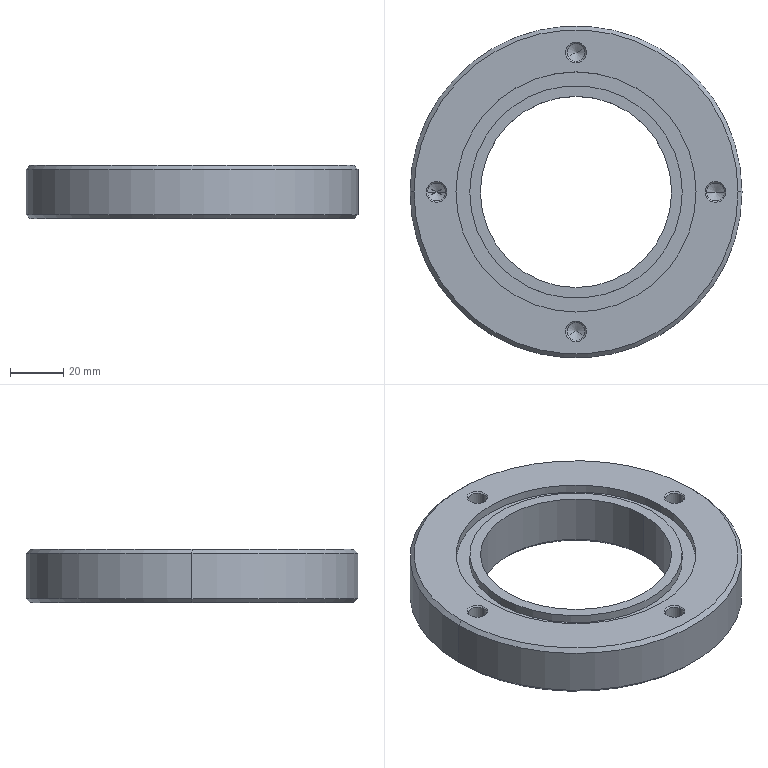Part | SolidWorks | features Chamfer 2, ICE 2, FlatPattern 1, HoleWzd 1, SMBaseFlange 1, SheetMetal 1 | 1 solid | 42 faces | box 125 x 125 x 20 mm | volume 156275 mm3 | cone 22 | cylinder 16 | plane 4 | commonest cylinder face diameters 6.8 x8 72 x2 80 x2 90.4 x2 125 x2
STEP:
#1=CARTESIAN_POINT('',(49.1,0.,-0.5));
#2=VERTEX_POINT('',#1);
#3=CARTESIAN_POINT('',(55.9,0.,-0.5));
#4=VERTEX_POINT('',#3);
#5=CARTESIAN_POINT('',(52.5,0.,-0.5));
#6=DIRECTION('',(0.,0.,1.));
#7=DIRECTION('',(1.,0.,0.));
#8=AXIS2_PLACEMENT_3D('',#5,#6,#7);
#9=CIRCLE('',#8,3.4);
#10=EDGE_CURVE('',#2,#4,#9,.T.);
#11=ORIENTED_EDGE('',*,*,#10,.F.);
#12=CARTESIAN_POINT('',(48.6,0.,0.));
#13=VERTEX_POINT('',#12);
#14=CARTESIAN_POINT('',(49.1,0.,-0.5));
#15=DIRECTION('',(-0.7071,0.,0.7071));
#16=VECTOR('',#15,1000.);
#17=LINE('',#14,#16);
#18=EDGE_CURVE('',#2,#13,#17,.T.);
#19=ORIENTED_EDGE('',*,*,#18,.T.);
#20=CARTESIAN_POINT('',(56.4,0.,0.));
#21=VERTEX_POINT('',#20);
#22=CARTESIAN_POINT('',(52.5,0.,0.));
#23=DIRECTION('',(0.,0.,-1.));
#24=DIRECTION('',(1.,0.,0.));
#25=AXIS2_PLACEMENT_3D('',#22,#23,#24);
#26=CIRCLE('',#25,3.9);
#27=EDGE_CURVE('',#21,#13,#26,.T.);
#28=ORIENTED_EDGE('',*,*,#27,.F.);
#29=CARTESIAN_POINT('',(55.9,0.,-0.5));
#30=DIRECTION('',(0.7071,0.,0.7071));
#31=VECTOR('',#30,1000.);
#32=LINE('',#29,#31);
#33=EDGE_CURVE('',#4,#21,#32,.T.);
#34=ORIENTED_EDGE('',*,*,#33,.F.);
#35=EDGE_LOOP('',(#11,#19,#28,#34));
#36=FACE_OUTER_BOUND('',#35,.T.);
#37=CARTESIAN_POINT('',(52.5,0.,-0.5));
#38=DIRECTION('',(0.,0.,1.));
#39=DIRECTION('',(1.,0.,0.));
#40=AXIS2_PLACEMENT_3D('',#37,#38,#39);
#41=CONICAL_SURFACE('',#40,3.4,0.7854);
#42=ADVANCED_FACE('',(#36),#41,.F.);
#43=CARTESIAN_POINT('',(-3.4,-52.5,-0.5));
#44=VERTEX_POINT('',#43);
#45=CARTESIAN_POINT('',(3.4,-52.5,-0.5));
#46=VERTEX_POINT('',#45);
#47=CARTESIAN_POINT('',(0.,-52.5,-0.5));
#48=DIRECTION('',(0.,0.,1.));
#49=DIRECTION('',(1.,0.,0.));
#50=AXIS2_PLACEMENT_3D('',#47,#48,#49);
#51=CIRCLE('',#50,3.4);
#52=EDGE_CURVE('',#44,#46,#51,.T.);
#53=ORIENTED_EDGE('',*,*,#52,.F.);
#54=CARTESIAN_POINT('',(-3.9,-52.5,0.));
#55=VERTEX_POINT('',#54);
#56=CARTESIAN_POINT('',(-3.4,-52.5,-0.5));
#57=DIRECTION('',(-0.7071,0.,0.7071));
#58=VECTOR('',#57,1000.);
#59=LINE('',#56,#58);
#60=EDGE_CURVE('',#44,#55,#59,.T.);
#61=ORIENTED_EDGE('',*,*,#60,.T.);
#62=CARTESIAN_POINT('',(3.9,-52.5,0.));
#63=VERTEX_POINT('',#62);
#64=CARTESIAN_POINT('',(0.,-52.5,0.));
#65=DIRECTION('',(0.,0.,-1.));
#66=DIRECTION('',(1.,0.,0.));
#67=AXIS2_PLACEMENT_3D('',#64,#65,#66);
#68=CIRCLE('',#67,3.9);
#69=EDGE_CURVE('',#63,#55,#68,.T.);
#70=ORIENTED_EDGE('',*,*,#69,.F.);
#71=CARTESIAN_POINT('',(3.4,-52.5,-0.5));
#72=DIRECTION('',(0.7071,0.,0.7071));
#73=VECTOR('',#72,1000.);
#74=LINE('',#71,#73);
#75=EDGE_CURVE('',#46,#63,#74,.T.);
#76=ORIENTED_EDGE('',*,*,#75,.F.);
#77=EDGE_LOOP('',(#53,#61,#70,#76));
#78=FACE_OUTER_BOUND('',#77,.T.);
#79=CARTESIAN_POINT('',(0.,-52.5,-0.5));
#80=DIRECTION('',(0.,0.,1.));
#81=DIRECTION('',(1.,0.,0.));
#82=AXIS2_PLACEMENT_3D('',#79,#80,#81);
#83=CONICAL_SURFACE('',#82,3.4,0.7854);
#84=ADVANCED_FACE('',(#78),#83,.F.);
#85=CARTESIAN_POINT('',(-55.9,0.,-0.5));
#86=VERTEX_POINT('',#85);
#87=CARTESIAN_POINT('',(-49.1,0.,-0.5));
#88=VERTEX_POINT('',#87);
#89=CARTESIAN_POINT('',(-52.5,0.,-0.5));
#90=DIRECTION('',(0.,0.,1.));
#91=DIRECTION('',(1.,0.,0.));
#92=AXIS2_PLACEMENT_3D('',#89,#90,#91);
#93=CIRCLE('',#92,3.4);
#94=EDGE_CURVE('',#86,#88,#93,.T.);
#95=ORIENTED_EDGE('',*,*,#94,.F.);
#96=CARTESIAN_POINT('',(-56.4,0.,0.));
#97=VERTEX_POINT('',#96);
#98=CARTESIAN_POINT('',(-55.9,0.,-0.5));
#99=DIRECTION('',(-0.7071,0.,0.7071));
#100=VECTOR('',#99,1000.);
#101=LINE('',#98,#100);
#102=EDGE_CURVE('',#86,#97,#101,.T.);
#103=ORIENTED_EDGE('',*,*,#102,.T.);
#104=CARTESIAN_POINT('',(-48.6,0.,0.));
#105=VERTEX_POINT('',#104);
#106=CARTESIAN_POINT('',(-52.5,0.,0.));
#107=DIRECTION('',(0.,0.,-1.));
#108=DIRECTION('',(1.,0.,0.));
#109=AXIS2_PLACEMENT_3D('',#106,#107,#108);
#110=CIRCLE('',#109,3.9);
#111=EDGE_CURVE('',#105,#97,#110,.T.);
#112=ORIENTED_EDGE('',*,*,#111,.F.);
#113=CARTESIAN_POINT('',(-49.1,0.,-0.5));
#114=DIRECTION('',(0.7071,0.,0.7071));
#115=VECTOR('',#114,1000.);
#116=LINE('',#113,#115);
#117=EDGE_CURVE('',#88,#105,#116,.T.);
#118=ORIENTED_EDGE('',*,*,#117,.F.);
#119=EDGE_LOOP('',(#95,#103,#112,#118));
#120=FACE_OUTER_BOUND('',#119,.T.);
#121=CARTESIAN_POINT('',(-52.5,0.,-0.5));
#122=DIRECTION('',(0.,0.,1.));
#123=DIRECTION('',(1.,0.,0.));
#124=AXIS2_PLACEMENT_3D('',#121,#122,#123);
#125=CONICAL_SURFACE('',#124,3.4,0.7854);
#126=ADVANCED_FACE('',(#120),#125,.F.);
#127=CARTESIAN_POINT('',(-3.4,52.5,-0.5));
#128=VERTEX_POINT('',#127);
#129=CARTESIAN_POINT('',(3.4,52.5,-0.5));
#130=VERTEX_POINT('',#129);
#131=CARTESIAN_POINT('',(0.,52.5,-0.5));
#132=DIRECTION('',(0.,0.,1.));
#133=DIRECTION('',(1.,0.,0.));
#134=AXIS2_PLACEMENT_3D('',#131,#132,#133);
#135=CIRCLE('',#134,3.4);
#136=EDGE_CURVE('',#128,#130,#135,.T.);
#137=ORIENTED_EDGE('',*,*,#136,.F.);
#138=CARTESIAN_POINT('',(-3.9,52.5,0.));
#139=VERTEX_POINT('',#138);
#140=CARTESIAN_POINT('',(-3.4,52.5,-0.5));
#141=DIRECTION('',(-0.7071,0.,0.7071));
#142=VECTOR('',#141,1000.);
#143=LINE('',#140,#142);
#144=EDGE_CURVE('',#128,#139,#143,.T.);
#145=ORIENTED_EDGE('',*,*,#144,.T.);
#146=CARTESIAN_POINT('',(3.9,52.5,0.));
#147=VERTEX_POINT('',#146);
#148=CARTESIAN_POINT('',(0.,52.5,0.));
#149=DIRECTION('',(0.,0.,-1.));
#150=DIRECTION('',(1.,0.,0.));
#151=AXIS2_PLACEMENT_3D('',#148,#149,#150);
#152=CIRCLE('',#151,3.9);
#153=EDGE_CURVE('',#147,#139,#152,.T.);
#154=ORIENTED_EDGE('',*,*,#153,.F.);
#155=CARTESIAN_POINT('',(3.4,52.5,-0.5));
#156=DIRECTION('',(0.7071,0.,0.7071));
#157=VECTOR('',#156,1000.);
#158=LINE('',#155,#157);
#159=EDGE_CURVE('',#130,#147,#158,.T.);
#160=ORIENTED_EDGE('',*,*,#159,.F.);
#161=EDGE_LOOP('',(#137,#145,#154,#160));
#162=FACE_OUTER_BOUND('',#161,.T.);
#163=CARTESIAN_POINT('',(0.,52.5,-0.5));
#164=DIRECTION('',(0.,0.,1.));
#165=DIRECTION('',(1.,0.,0.));
#166=AXIS2_PLACEMENT_3D('',#163,#164,#165);
#167=CONICAL_SURFACE('',#166,3.4,0.7854);
#168=ADVANCED_FACE('',(#162),#167,.F.);
#169=CARTESIAN_POINT('',(61.,0.,0.));
#170=VERTEX_POINT('',#169);
#171=CARTESIAN_POINT('',(-61.,0.,0.));
#172=VERTEX_POINT('',#171);
#173=CARTESIAN_POINT('',(0.,0.,0.));
#174=DIRECTION('',(0.,0.,1.));
#175=DIRECTION('',(1.,0.,0.));
#176=AXIS2_PLACEMENT_3D('',#173,#174,#175);
#177=CIRCLE('',#176,61.);
#178=EDGE_CURVE('',#170,#172,#177,.T.);
#179=ORIENTED_EDGE('',*,*,#178,.F.);
#180=CARTESIAN_POINT('',(62.5,0.,-1.5));
#181=VERTEX_POINT('',#180);
#182=CARTESIAN_POINT('',(61.,0.,0.));
#183=DIRECTION('',(0.7071,0.,-0.7071));
#184=VECTOR('',#183,1000.);
#185=LINE('',#182,#184);
#186=EDGE_CURVE('',#170,#181,#185,.T.);
#187=ORIENTED_EDGE('',*,*,#186,.T.);
#188=CARTESIAN_POINT('',(-62.5,0.,-1.5));
#189=VERTEX_POINT('',#188);
#190=CARTESIAN_POINT('',(0.,0.,-1.5));
#191=DIRECTION('',(0.,0.,-1.));
#192=DIRECTION('',(1.,0.,0.));
#193=AXIS2_PLACEMENT_3D('',#190,#191,#192);
#194=CIRCLE('',#193,62.5);
#195=EDGE_CURVE('',#189,#181,#194,.T.);
#196=ORIENTED_EDGE('',*,*,#195,.F.);
#197=CARTESIAN_POINT('',(-61.,0.,0.));
#198=DIRECTION('',(-0.7071,0.,-0.7071));
#199=VECTOR('',#198,1000.);
#200=LINE('',#197,#199);
#201=EDGE_CURVE('',#172,#189,#200,.T.);
#202=ORIENTED_EDGE('',*,*,#201,.F.);
#203=EDGE_LOOP('',(#179,#187,#196,#202));
#204=FACE_OUTER_BOUND('',#203,.T.);
#205=CARTESIAN_POINT('',(0.,0.,0.));
#206=DIRECTION('',(0.,0.,-1.));
#207=DIRECTION('',(-1.,0.,0.));
#208=AXIS2_PLACEMENT_3D('',#205,#206,#207);
#209=CONICAL_SURFACE('',#208,61.,0.7854);
#210=ADVANCED_FACE('',(#204),#209,.T.);
#211=CARTESIAN_POINT('',(-61.,0.,-20.));
#212=VERTEX_POINT('',#211);
#213=CARTESIAN_POINT('',(61.,0.,-20.));
#214=VERTEX_POINT('',#213);
#215=CARTESIAN_POINT('',(0.,0.,-20.));
#216=DIRECTION('',(0.,0.,-1.));
#217=DIRECTION('',(1.,0.,0.));
#218=AXIS2_PLACEMENT_3D('',#215,#216,#217);
#219=CIRCLE('',#218,61.);
#220=EDGE_CURVE('',#212,#214,#219,.T.);
#221=ORIENTED_EDGE('',*,*,#220,.F.);
#222=CARTESIAN_POINT('',(-62.5,0.,-18.5));
#223=VERTEX_POINT('',#222);
#224=CARTESIAN_POINT('',(-62.5,0.,-18.5));
#225=DIRECTION('',(-0.7071,0.,0.7071));
#226=VECTOR('',#225,1000.);
#227=LINE('',#224,#226);
#228=EDGE_CURVE('',#212,#223,#227,.T.);
#229=ORIENTED_EDGE('',*,*,#228,.T.);
#230=CARTESIAN_POINT('',(62.5,0.,-18.5));
#231=VERTEX_POINT('',#230);
#232=CARTESIAN_POINT('',(0.,0.,-18.5));
#233=DIRECTION('',(0.,0.,1.));
#234=DIRECTION('',(1.,0.,0.));
#235=AXIS2_PLACEMENT_3D('',#232,#233,#234);
#236=CIRCLE('',#235,62.5);
#237=EDGE_CURVE('',#231,#223,#236,.T.);
#238=ORIENTED_EDGE('',*,*,#237,.F.);
#239=CARTESIAN_POINT('',(62.5,0.,-18.5));
#240=DIRECTION('',(0.7071,0.,0.7071));
#241=VECTOR('',#240,1000.);
#242=LINE('',#239,#241);
#243=EDGE_CURVE('',#214,#231,#242,.T.);
#244=ORIENTED_EDGE('',*,*,#243,.F.);
#245=EDGE_LOOP('',(#221,#229,#238,#244));
#246=FACE_OUTER_BOUND('',#245,.T.);
#247=CARTESIAN_POINT('',(0.,0.,-18.5));
#248=DIRECTION('',(0.,0.,1.));
#249=DIRECTION('',(1.,0.,0.));
#250=AXIS2_PLACEMENT_3D('',#247,#248,#249);
#251=CONICAL_SURFACE('',#250,62.5,0.7854);
#252=ADVANCED_FACE('',(#246),#251,.T.);
#253=CARTESIAN_POINT('',(36.,0.,-18.5));
#254=VERTEX_POINT('',#253);
#255=CARTESIAN_POINT('',(-36.,0.,-18.5));
#256=VERTEX_POINT('',#255);
#257=CARTESIAN_POINT('',(0.,0.,-18.5));
#258=DIRECTION('',(0.,0.,-1.));
#259=DIRECTION('',(1.,0.,0.));
#260=AXIS2_PLACEMENT_3D('',#257,#258,#259);
#261=CIRCLE('',#260,36.);
#262=EDGE_CURVE('',#254,#256,#261,.T.);
#263=ORIENTED_EDGE('',*,*,#262,.F.);
#264=CARTESIAN_POINT('',(37.5,0.,-20.));
#265=VERTEX_POINT('',#264);
#266=CARTESIAN_POINT('',(37.5,0.,-20.));
#267=DIRECTION('',(0.7071,0.,-0.7071));
#268=VECTOR('',#267,1000.);
#269=LINE('',#266,#268);
#270=EDGE_CURVE('',#254,#265,#269,.T.);
#271=ORIENTED_EDGE('',*,*,#270,.T.);
#272=CARTESIAN_POINT('',(-37.5,0.,-20.));
#273=VERTEX_POINT('',#272);
#274=CARTESIAN_POINT('',(0.,0.,-20.));
#275=DIRECTION('',(0.,0.,1.));
#276=DIRECTION('',(1.,0.,0.));
#277=AXIS2_PLACEMENT_3D('',#274,#275,#276);
#278=CIRCLE('',#277,37.5);
#279=EDGE_CURVE('',#273,#265,#278,.T.);
#280=ORIENTED_EDGE('',*,*,#279,.F.);
#281=CARTESIAN_POINT('',(-37.5,0.,-20.));
#282=DIRECTION('',(-0.7071,0.,-0.7071));
#283=VECTOR('',#282,1000.);
#284=LINE('',#281,#283);
#285=EDGE_CURVE('',#256,#273,#284,.T.);
#286=ORIENTED_EDGE('',*,*,#285,.F.);
#287=EDGE_LOOP('',(#263,#271,#280,#286));
#288=FACE_OUTER_BOUND('',#287,.T.);
#289=CARTESIAN_POINT('',(0.,0.,-20.));
#290=DIRECTION('',(0.,0.,-1.));
#291=DIRECTION('',(-1.,0.,0.));
#292=AXIS2_PLACEMENT_3D('',#289,#290,#291);
#293=CONICAL_SURFACE('',#292,37.5,0.7854);
#294=ADVANCED_FACE('',(#288),#293,.F.);
#295=CARTESIAN_POINT('',(-3.4,52.5,-14.));
#296=VERTEX_POINT('',#295);
#297=CARTESIAN_POINT('',(3.4,52.5,-14.));
#298=VERTEX_POINT('',#297);
#299=CARTESIAN_POINT('',(0.,52.5,-14.));
#300=DIRECTION('',(0.,0.,1.));
#301=DIRECTION('',(1.,0.,0.));
#302=AXIS2_PLACEMENT_3D('',#299,#300,#301);
#303=CIRCLE('',#302,3.4);
#304=EDGE_CURVE('',#296,#298,#303,.T.);
#305=ORIENTED_EDGE('',*,*,#304,.F.);
#306=CARTESIAN_POINT('',(-3.4,52.5,0.));
#307=DIRECTION('',(0.,0.,1.));
#308=VECTOR('',#307,1000.);
#309=LINE('',#306,#308);
#310=EDGE_CURVE('',#296,#128,#309,.T.);
#311=ORIENTED_EDGE('',*,*,#310,.T.);
#312=ORIENTED_EDGE('',*,*,#136,.T.);
#313=CARTESIAN_POINT('',(3.4,52.5,0.));
#314=DIRECTION('',(0.,0.,1.));
#315=VECTOR('',#314,1000.);
#316=LINE('',#313,#315);
#317=EDGE_CURVE('',#298,#130,#316,.T.);
#318=ORIENTED_EDGE('',*,*,#317,.F.);
#319=EDGE_LOOP('',(#305,#311,#312,#318));
#320=FACE_OUTER_BOUND('',#319,.T.);
#321=CARTESIAN_POINT('',(0.,52.5,0.));
#322=DIRECTION('',(0.,0.,1.));
#323=DIRECTION('',(1.,0.,0.));
#324=AXIS2_PLACEMENT_3D('',#321,#322,#323);
#325=CYLINDRICAL_SURFACE('',#324,3.4);
#326=ADVANCED_FACE('',(#320),#325,.F.);
#327=CARTESIAN_POINT('',(0.,52.5,-16.043));
#328=VERTEX_POINT('',#327);
#329=CARTESIAN_POINT('',(3.4,52.5,-14.));
#330=DIRECTION('',(0.8572,0.,0.515));
#331=VECTOR('',#330,1000.);
#332=LINE('',#329,#331);
#333=EDGE_CURVE('',#328,#298,#332,.T.);
#334=ORIENTED_EDGE('',*,*,#333,.F.);
#335=CARTESIAN_POINT('',(-3.4,52.5,-14.));
#336=DIRECTION('',(-0.8572,0.,0.515));
#337=VECTOR('',#336,1000.);
#338=LINE('',#335,#337);
#339=EDGE_CURVE('',#328,#296,#338,.T.);
#340=ORIENTED_EDGE('',*,*,#339,.T.);
#341=ORIENTED_EDGE('',*,*,#304,.T.);
#342=EDGE_LOOP('',(#334,#340,#341));
#343=FACE_OUTER_BOUND('',#342,.T.);
#344=CARTESIAN_POINT('',(0.,52.5,-14.));
#345=DIRECTION('',(0.,0.,1.));
#346=DIRECTION('',(1.,0.,0.));
#347=AXIS2_PLACEMENT_3D('',#344,#345,#346);
#348=CONICAL_SURFACE('',#347,3.4,1.03);
#349=ADVANCED_FACE('',(#343),#348,.F.);
#350=CARTESIAN_POINT('',(49.1,0.,-14.));
#351=VERTEX_POINT('',#350);
#352=CARTESIAN_POINT('',(55.9,0.,-14.));
#353=VERTEX_POINT('',#352);
#354=CARTESIAN_POINT('',(52.5,0.,-14.));
#355=DIRECTION('',(0.,0.,1.));
#356=DIRECTION('',(1.,0.,0.));
#357=AXIS2_PLACEMENT_3D('',#354,#355,#356);
#358=CIRCLE('',#357,3.4);
#359=EDGE_CURVE('',#351,#353,#358,.T.);
#360=ORIENTED_EDGE('',*,*,#359,.F.);
#361=CARTESIAN_POINT('',(49.1,0.,0.));
#362=DIRECTION('',(0.,0.,1.));
#363=VECTOR('',#362,1000.);
#364=LINE('',#361,#363);
#365=EDGE_CURVE('',#351,#2,#364,.T.);
#366=ORIENTED_EDGE('',*,*,#365,.T.);
#367=ORIENTED_EDGE('',*,*,#10,.T.);
#368=CARTESIAN_POINT('',(55.9,0.,0.));
#369=DIRECTION('',(0.,0.,1.));
#370=VECTOR('',#369,1000.);
#371=LINE('',#368,#370);
#372=EDGE_CURVE('',#353,#4,#371,.T.);
#373=ORIENTED_EDGE('',*,*,#372,.F.);
#374=EDGE_LOOP('',(#360,#366,#367,#373));
#375=FACE_OUTER_BOUND('',#374,.T.);
#376=CARTESIAN_POINT('',(52.5,0.,0.));
#377=DIRECTION('',(0.,0.,1.));
#378=DIRECTION('',(1.,0.,0.));
#379=AXIS2_PLACEMENT_3D('',#376,#377,#378);
#380=CYLINDRICAL_SURFACE('',#379,3.4);
#381=ADVANCED_FACE('',(#375),#380,.F.);
#382=CARTESIAN_POINT('',(52.5,0.,-16.043));
#383=VERTEX_POINT('',#382);
#384=CARTESIAN_POINT('',(55.9,0.,-14.));
#385=DIRECTION('',(0.8572,0.,0.515));
#386=VECTOR('',#385,1000.);
#387=LINE('',#384,#386);
#388=EDGE_CURVE('',#383,#353,#387,.T.);
#389=ORIENTED_EDGE('',*,*,#388,.F.);
#390=CARTESIAN_POINT('',(49.1,0.,-14.));
#391=DIRECTION('',(-0.8572,0.,0.515));
#392=VECTOR('',#391,1000.);
#393=LINE('',#390,#392);
#394=EDGE_CURVE('',#383,#351,#393,.T.);
#395=ORIENTED_EDGE('',*,*,#394,.T.);
#396=ORIENTED_EDGE('',*,*,#359,.T.);
#397=EDGE_LOOP('',(#389,#395,#396));
#398=FACE_OUTER_BOUND('',#397,.T.);
#399=CARTESIAN_POINT('',(52.5,0.,-14.));
#400=DIRECTION('',(0.,0.,1.));
#401=DIRECTION('',(1.,0.,0.));
#402=AXIS2_PLACEMENT_3D('',#399,#400,#401);
#403=CONICAL_SURFACE('',#402,3.4,1.03);
#404=ADVANCED_FACE('',(#398),#403,.F.);
#405=CARTESIAN_POINT('',(-3.4,-52.5,-14.));
#406=VERTEX_POINT('',#405);
#407=CARTESIAN_POINT('',(3.4,-52.5,-14.));
#408=VERTEX_POINT('',#407);
#409=CARTESIAN_POINT('',(0.,-52.5,-14.));
#410=DIRECTION('',(0.,0.,1.));
#411=DIRECTION('',(1.,0.,0.));
#412=AXIS2_PLACEMENT_3D('',#409,#410,#411);
#413=CIRCLE('',#412,3.4);
#414=EDGE_CURVE('',#406,#408,#413,.T.);
#415=ORIENTED_EDGE('',*,*,#414,.F.);
#416=CARTESIAN_POINT('',(-3.4,-52.5,0.));
#417=DIRECTION('',(0.,0.,1.));
#418=VECTOR('',#417,1000.);
#419=LINE('',#416,#418);
#420=EDGE_CURVE('',#406,#44,#419,.T.);
#421=ORIENTED_EDGE('',*,*,#420,.T.);
#422=ORIENTED_EDGE('',*,*,#52,.T.);
#423=CARTESIAN_POINT('',(3.4,-52.5,0.));
#424=DIRECTION('',(0.,0.,1.));
#425=VECTOR('',#424,1000.);
#426=LINE('',#423,#425);
#427=EDGE_CURVE('',#408,#46,#426,.T.);
#428=ORIENTED_EDGE('',*,*,#427,.F.);
#429=EDGE_LOOP('',(#415,#421,#422,#428));
#430=FACE_OUTER_BOUND('',#429,.T.);
#431=CARTESIAN_POINT('',(0.,-52.5,0.));
#432=DIRECTION('',(0.,0.,1.));
#433=DIRECTION('',(1.,0.,0.));
#434=AXIS2_PLACEMENT_3D('',#431,#432,#433);
#435=CYLINDRICAL_SURFACE('',#434,3.4);
#436=ADVANCED_FACE('',(#430),#435,.F.);
#437=CARTESIAN_POINT('',(0.,-52.5,-16.043));
#438=VERTEX_POINT('',#437);
#439=CARTESIAN_POINT('',(3.4,-52.5,-14.));
#440=DIRECTION('',(0.8572,0.,0.515));
#441=VECTOR('',#440,1000.);
#442=LINE('',#439,#441);
#443=EDGE_CURVE('',#438,#408,#442,.T.);
#444=ORIENTED_EDGE('',*,*,#443,.F.);
#445=CARTESIAN_POINT('',(-3.4,-52.5,-14.));
#446=DIRECTION('',(-0.8572,0.,0.515));
#447=VECTOR('',#446,1000.);
#448=LINE('',#445,#447);
#449=EDGE_CURVE('',#438,#406,#448,.T.);
#450=ORIENTED_EDGE('',*,*,#449,.T.);
#451=ORIENTED_EDGE('',*,*,#414,.T.);
#452=EDGE_LOOP('',(#444,#450,#451));
#453=FACE_OUTER_BOUND('',#452,.T.);
#454=CARTESIAN_POINT('',(0.,-52.5,-14.));
#455=DIRECTION('',(0.,0.,1.));
#456=DIRECTION('',(1.,0.,0.));
#457=AXIS2_PLACEMENT_3D('',#454,#455,#456);
#458=CONICAL_SURFACE('',#457,3.4,1.03);
#459=ADVANCED_FACE('',(#453),#458,.F.);
#460=CARTESIAN_POINT('',(-55.9,0.,-14.));
#461=VERTEX_POINT('',#460);
#462=CARTESIAN_POINT('',(-49.1,0.,-14.));
#463=VERTEX_POINT('',#462);
#464=CARTESIAN_POINT('',(-52.5,0.,-14.));
#465=DIRECTION('',(0.,0.,1.));
#466=DIRECTION('',(1.,0.,0.));
#467=AXIS2_PLACEMENT_3D('',#464,#465,#466);
#468=CIRCLE('',#467,3.4);
#469=EDGE_CURVE('',#461,#463,#468,.T.);
#470=ORIENTED_EDGE('',*,*,#469,.F.);
#471=CARTESIAN_POINT('',(-55.9,0.,0.));
#472=DIRECTION('',(0.,0.,1.));
#473=VECTOR('',#472,1000.);
#474=LINE('',#471,#473);
#475=EDGE_CURVE('',#461,#86,#474,.T.);
#476=ORIENTED_EDGE('',*,*,#475,.T.);
#477=ORIENTED_EDGE('',*,*,#94,.T.);
#478=CARTESIAN_POINT('',(-49.1,0.,0.));
#479=DIRECTION('',(0.,0.,1.));
#480=VECTOR('',#479,1000.);
#481=LINE('',#478,#480);
#482=EDGE_CURVE('',#463,#88,#481,.T.);
#483=ORIENTED_EDGE('',*,*,#482,.F.);
#484=EDGE_LOOP('',(#470,#476,#477,#483));
#485=FACE_OUTER_BOUND('',#484,.T.);
#486=CARTESIAN_POINT('',(-52.5,0.,0.));
#487=DIRECTION('',(0.,0.,1.));
#488=DIRECTION('',(1.,0.,0.));
#489=AXIS2_PLACEMENT_3D('',#486,#487,#488);
#490=CYLINDRICAL_SURFACE('',#489,3.4);
#491=ADVANCED_FACE('',(#485),#490,.F.);
#492=CARTESIAN_POINT('',(-52.5,0.,-16.043));
#493=VERTEX_POINT('',#492);
#494=CARTESIAN_POINT('',(-49.1,0.,-14.));
#495=DIRECTION('',(0.8572,0.,0.515));
#496=VECTOR('',#495,1000.);
#497=LINE('',#494,#496);
#498=EDGE_CURVE('',#493,#463,#497,.T.);
#499=ORIENTED_EDGE('',*,*,#498,.F.);
#500=CARTESIAN_POINT('',(-55.9,0.,-14.));
#501=DIRECTION('',(-0.8572,0.,0.515));
#502=VECTOR('',#501,1000.);
#503=LINE('',#500,#502);
#504=EDGE_CURVE('',#493,#461,#503,.T.);
#505=ORIENTED_EDGE('',*,*,#504,.T.);
#506=ORIENTED_EDGE('',*,*,#469,.T.);
#507=EDGE_LOOP('',(#499,#505,#506));
#508=FACE_OUTER_BOUND('',#507,.T.);
#509=CARTESIAN_POINT('',(-52.5,0.,-14.));
#510=DIRECTION('',(0.,0.,1.));
#511=DIRECTION('',(1.,0.,0.));
#512=AXIS2_PLACEMENT_3D('',#509,#510,#511);
#513=CONICAL_SURFACE('',#512,3.4,1.03);
#514=ADVANCED_FACE('',(#508),#513,.F.);
#515=CARTESIAN_POINT('',(40.,0.,-3.2));
#516=VERTEX_POINT('',#515);
#517=CARTESIAN_POINT('',(-40.,0.,-3.2));
#518=VERTEX_POINT('',#517);
#519=CARTESIAN_POINT('',(0.,0.,-3.2));
#520=DIRECTION('',(0.,0.,1.));
#521=DIRECTION('',(1.,0.,0.));
#522=AXIS2_PLACEMENT_3D('',#519,#520,#521);
#523=CIRCLE('',#522,40.);
#524=EDGE_CURVE('',#516,#518,#523,.T.);
#525=ORIENTED_EDGE('',*,*,#524,.T.);
#526=CARTESIAN_POINT('',(-40.,0.,0.));
#527=VERTEX_POINT('',#526);
#528=CARTESIAN_POINT('',(-40.,0.,-3.2));
#529=DIRECTION('',(0.,0.,1.));
#530=VECTOR('',#529,1000.);
#531=LINE('',#528,#530);
#532=EDGE_CURVE('',#518,#527,#531,.T.);
#533=ORIENTED_EDGE('',*,*,#532,.T.);
#534=CARTESIAN_POINT('',(40.,0.,0.));
#535=VERTEX_POINT('',#534);
#536=CARTESIAN_POINT('',(0.,0.,0.));
#537=DIRECTION('',(0.,0.,1.));
#538=DIRECTION('',(1.,0.,0.));
#539=AXIS2_PLACEMENT_3D('',#536,#537,#538);
#540=CIRCLE('',#539,40.);
#541=EDGE_CURVE('',#535,#527,#540,.T.);
#542=ORIENTED_EDGE('',*,*,#541,.F.);
#543=CARTESIAN_POINT('',(40.,0.,-3.2));
#544=DIRECTION('',(0.,0.,1.));
#545=VECTOR('',#544,1000.);
#546=LINE('',#543,#545);
#547=EDGE_CURVE('',#516,#535,#546,.T.);
#548=ORIENTED_EDGE('',*,*,#547,.F.);
#549=EDGE_LOOP('',(#525,#533,#542,#548));
#550=FACE_OUTER_BOUND('',#549,.T.);
#551=CARTESIAN_POINT('',(0.,0.,-3.2));
#552=DIRECTION('',(0.,0.,1.));
#553=DIRECTION('',(1.,0.,0.));
#554=AXIS2_PLACEMENT_3D('',#551,#552,#553);
#555=CYLINDRICAL_SURFACE('',#554,40.);
#556=ADVANCED_FACE('',(#550),#555,.T.);
#557=CARTESIAN_POINT('',(-45.2,0.,-3.2));
#558=VERTEX_POINT('',#557);
#559=CARTESIAN_POINT('',(45.2,0.,-3.2));
#560=VERTEX_POINT('',#559);
#561=CARTESIAN_POINT('',(0.,0.,-3.2));
#562=DIRECTION('',(0.,0.,1.));
#563=DIRECTION('',(1.,0.,0.));
#564=AXIS2_PLACEMENT_3D('',#561,#562,#563);
#565=CIRCLE('',#564,45.2);
#566=EDGE_CURVE('',#558,#560,#565,.T.);
#567=ORIENTED_EDGE('',*,*,#566,.F.);
#568=CARTESIAN_POINT('',(-45.2,0.,0.));
#569=VERTEX_POINT('',#568);
#570=CARTESIAN_POINT('',(-45.2,0.,-3.2));
#571=DIRECTION('',(0.,0.,1.));
#572=VECTOR('',#571,1000.);
#573=LINE('',#570,#572);
#574=EDGE_CURVE('',#558,#569,#573,.T.);
#575=ORIENTED_EDGE('',*,*,#574,.T.);
#576=CARTESIAN_POINT('',(45.2,0.,0.));
#577=VERTEX_POINT('',#576);
#578=CARTESIAN_POINT('',(0.,0.,0.));
#579=DIRECTION('',(0.,0.,1.));
#580=DIRECTION('',(1.,0.,0.));
#581=AXIS2_PLACEMENT_3D('',#578,#579,#580);
#582=CIRCLE('',#581,45.2);
#583=EDGE_CURVE('',#569,#577,#582,.T.);
#584=ORIENTED_EDGE('',*,*,#583,.T.);
#585=CARTESIAN_POINT('',(45.2,0.,-3.2));
#586=DIRECTION('',(0.,0.,1.));
#587=VECTOR('',#586,1000.);
#588=LINE('',#585,#587);
#589=EDGE_CURVE('',#560,#577,#588,.T.);
#590=ORIENTED_EDGE('',*,*,#589,.F.);
#591=EDGE_LOOP('',(#567,#575,#584,#590));
#592=FACE_OUTER_BOUND('',#591,.T.);
#593=CARTESIAN_POINT('',(0.,0.,-3.2));
#594=DIRECTION('',(0.,0.,1.));
#595=DIRECTION('',(1.,0.,0.));
#596=AXIS2_PLACEMENT_3D('',#593,#594,#595);
#597=CYLINDRICAL_SURFACE('',#596,45.2);
#598=ADVANCED_FACE('',(#592),#597,.F.);
#599=ORIENTED_EDGE('',*,*,#262,.T.);
#600=CARTESIAN_POINT('',(-36.,0.,0.));
#601=VERTEX_POINT('',#600);
#602=CARTESIAN_POINT('',(-36.,0.,-20.));
#603=DIRECTION('',(0.,0.,1.));
#604=VECTOR('',#603,1000.);
#605=LINE('',#602,#604);
#606=EDGE_CURVE('',#256,#601,#605,.T.);
#607=ORIENTED_EDGE('',*,*,#606,.T.);
#608=CARTESIAN_POINT('',(36.,0.,0.));
#609=VERTEX_POINT('',#608);
#610=CARTESIAN_POINT('',(0.,0.,0.));
#611=DIRECTION('',(0.,0.,1.));
#612=DIRECTION('',(1.,0.,0.));
#613=AXIS2_PLACEMENT_3D('',#610,#611,#612);
#614=CIRCLE('',#613,36.);
#615=EDGE_CURVE('',#601,#609,#614,.T.);
#616=ORIENTED_EDGE('',*,*,#615,.T.);
#617=CARTESIAN_POINT('',(36.,0.,-20.));
#618=DIRECTION('',(0.,0.,1.));
#619=VECTOR('',#618,1000.);
#620=LINE('',#617,#619);
#621=EDGE_CURVE('',#254,#609,#620,.T.);
#622=ORIENTED_EDGE('',*,*,#621,.F.);
#623=EDGE_LOOP('',(#599,#607,#616,#622));
#624=FACE_OUTER_BOUND('',#623,.T.);
#625=CARTESIAN_POINT('',(0.,0.,-20.));
#626=DIRECTION('',(0.,0.,1.));
#627=DIRECTION('',(1.,0.,0.));
#628=AXIS2_PLACEMENT_3D('',#625,#626,#627);
#629=CYLINDRICAL_SURFACE('',#628,36.);
#630=ADVANCED_FACE('',(#624),#629,.F.);
#631=ORIENTED_EDGE('',*,*,#237,.T.);
#632=CARTESIAN_POINT('',(-62.5,0.,-20.));
#633=DIRECTION('',(0.,0.,1.));
#634=VECTOR('',#633,1000.);
#635=LINE('',#632,#634);
#636=EDGE_CURVE('',#223,#189,#635,.T.);
#637=ORIENTED_EDGE('',*,*,#636,.T.);
#638=ORIENTED_EDGE('',*,*,#195,.T.);
#639=CARTESIAN_POINT('',(62.5,0.,-20.));
#640=DIRECTION('',(0.,0.,1.));
#641=VECTOR('',#640,1000.);
#642=LINE('',#639,#641);
#643=EDGE_CURVE('',#231,#181,#642,.T.);
#644=ORIENTED_EDGE('',*,*,#643,.F.);
#645=EDGE_LOOP('',(#631,#637,#638,#644));
#646=FACE_OUTER_BOUND('',#645,.T.);
#647=CARTESIAN_POINT('',(0.,0.,-20.));
#648=DIRECTION('',(0.,0.,1.));
#649=DIRECTION('',(1.,0.,0.));
#650=AXIS2_PLACEMENT_3D('',#647,#648,#649);
#651=CYLINDRICAL_SURFACE('',#650,62.5);
#652=ADVANCED_FACE('',(#646),#651,.T.);
#653=CARTESIAN_POINT('',(0.,0.,0.));
#654=DIRECTION('',(0.,0.,1.));
#655=DIRECTION('',(1.,0.,0.));
#656=AXIS2_PLACEMENT_3D('',#653,#654,#655);
#657=CIRCLE('',#656,36.);
#658=EDGE_CURVE('',#609,#601,#657,.T.);
#659=ORIENTED_EDGE('',*,*,#658,.F.);
#660=ORIENTED_EDGE('',*,*,#615,.F.);
#661=EDGE_LOOP('',(#659,#660));
#662=FACE_BOUND('',#661,.T.);
#663=ORIENTED_EDGE('',*,*,#541,.T.);
#664=CARTESIAN_POINT('',(0.,0.,0.));
#665=DIRECTION('',(0.,0.,1.));
#666=DIRECTION('',(1.,0.,0.));
#667=AXIS2_PLACEMENT_3D('',#664,#665,#666);
#668=CIRCLE('',#667,40.);
#669=EDGE_CURVE('',#527,#535,#668,.T.);
#670=ORIENTED_EDGE('',*,*,#669,.T.);
#671=EDGE_LOOP('',(#663,#670));
#672=FACE_OUTER_BOUND('',#671,.T.);
#673=CARTESIAN_POINT('',(0.,0.,0.));
#674=DIRECTION('',(0.,0.,1.));
#675=DIRECTION('',(1.,0.,0.));
#676=AXIS2_PLACEMENT_3D('',#673,#674,#675);
#677=PLANE('',#676);
#678=ADVANCED_FACE('',(#662,#672),#677,.T.);
#679=ORIENTED_EDGE('',*,*,#636,.F.);
#680=CARTESIAN_POINT('',(0.,0.,-18.5));
#681=DIRECTION('',(0.,0.,1.));
#682=DIRECTION('',(1.,0.,0.));
#683=AXIS2_PLACEMENT_3D('',#680,#681,#682);
#684=CIRCLE('',#683,62.5);
#685=EDGE_CURVE('',#223,#231,#684,.T.);
#686=ORIENTED_EDGE('',*,*,#685,.T.);
#687=ORIENTED_EDGE('',*,*,#643,.T.);
#688=CARTESIAN_POINT('',(0.,0.,-1.5));
#689=DIRECTION('',(0.,0.,-1.));
#690=DIRECTION('',(1.,0.,0.));
#691=AXIS2_PLACEMENT_3D('',#688,#689,#690);
#692=CIRCLE('',#691,62.5);
#693=EDGE_CURVE('',#181,#189,#692,.T.);
#694=ORIENTED_EDGE('',*,*,#693,.T.);
#695=EDGE_LOOP('',(#679,#686,#687,#694));
#696=FACE_OUTER_BOUND('',#695,.T.);
#697=CARTESIAN_POINT('',(0.,0.,-20.));
#698=DIRECTION('',(0.,0.,1.));
#699=DIRECTION('',(1.,0.,0.));
#700=AXIS2_PLACEMENT_3D('',#697,#698,#699);
#701=CYLINDRICAL_SURFACE('',#700,62.5);
#702=ADVANCED_FACE('',(#696),#701,.T.);
#703=ORIENTED_EDGE('',*,*,#279,.T.);
#704=CARTESIAN_POINT('',(0.,0.,-20.));
#705=DIRECTION('',(0.,0.,1.));
#706=DIRECTION('',(1.,0.,0.));
#707=AXIS2_PLACEMENT_3D('',#704,#705,#706);
#708=CIRCLE('',#707,37.5);
#709=EDGE_CURVE('',#265,#273,#708,.T.);
#710=ORIENTED_EDGE('',*,*,#709,.T.);
#711=EDGE_LOOP('',(#703,#710));
#712=FACE_BOUND('',#711,.T.);
#713=CARTESIAN_POINT('',(0.,0.,-20.));
#714=DIRECTION('',(0.,0.,-1.));
#715=DIRECTION('',(1.,0.,0.));
#716=AXIS2_PLACEMENT_3D('',#713,#714,#715);
#717=CIRCLE('',#716,61.);
#718=EDGE_CURVE('',#214,#212,#717,.T.);
#719=ORIENTED_EDGE('',*,*,#718,.T.);
#720=ORIENTED_EDGE('',*,*,#220,.T.);
#721=EDGE_LOOP('',(#719,#720));
#722=FACE_OUTER_BOUND('',#721,.T.);
#723=CARTESIAN_POINT('',(0.,0.,-20.));
#724=DIRECTION('',(0.,0.,1.));
#725=DIRECTION('',(1.,0.,0.));
#726=AXIS2_PLACEMENT_3D('',#723,#724,#725);
#727=PLANE('',#726);
#728=ADVANCED_FACE('',(#712,#722),#727,.F.);
#729=ORIENTED_EDGE('',*,*,#153,.T.);
#730=CARTESIAN_POINT('',(0.,52.5,0.));
#731=DIRECTION('',(0.,0.,-1.));
#732=DIRECTION('',(1.,0.,0.));
#733=AXIS2_PLACEMENT_3D('',#730,#731,#732);
#734=CIRCLE('',#733,3.9);
#735=EDGE_CURVE('',#139,#147,#734,.T.);
#736=ORIENTED_EDGE('',*,*,#735,.T.);
#737=EDGE_LOOP('',(#729,#736));
#738=FACE_BOUND('',#737,.T.);
#739=ORIENTED_EDGE('',*,*,#111,.T.);
#740=CARTESIAN_POINT('',(-52.5,0.,0.));
#741=DIRECTION('',(0.,0.,-1.));
#742=DIRECTION('',(1.,0.,0.));
#743=AXIS2_PLACEMENT_3D('',#740,#741,#742);
#744=CIRCLE('',#743,3.9);
#745=EDGE_CURVE('',#97,#105,#744,.T.);
#746=ORIENTED_EDGE('',*,*,#745,.T.);
#747=EDGE_LOOP('',(#739,#746));
#748=FACE_BOUND('',#747,.T.);
#749=ORIENTED_EDGE('',*,*,#69,.T.);
#750=CARTESIAN_POINT('',(0.,-52.5,0.));
#751=DIRECTION('',(0.,0.,-1.));
#752=DIRECTION('',(1.,0.,0.));
#753=AXIS2_PLACEMENT_3D('',#750,#751,#752);
#754=CIRCLE('',#753,3.9);
#755=EDGE_CURVE('',#55,#63,#754,.T.);
#756=ORIENTED_EDGE('',*,*,#755,.T.);
#757=EDGE_LOOP('',(#749,#756));
#758=FACE_BOUND('',#757,.T.);
#759=ORIENTED_EDGE('',*,*,#27,.T.);
#760=CARTESIAN_POINT('',(52.5,0.,0.));
#761=DIRECTION('',(0.,0.,-1.));
#762=DIRECTION('',(1.,0.,0.));
#763=AXIS2_PLACEMENT_3D('',#760,#761,#762);
#764=CIRCLE('',#763,3.9);
#765=EDGE_CURVE('',#13,#21,#764,.T.);
#766=ORIENTED_EDGE('',*,*,#765,.T.);
#767=EDGE_LOOP('',(#759,#766));
#768=FACE_BOUND('',#767,.T.);
#769=CARTESIAN_POINT('',(0.,0.,0.));
#770=DIRECTION('',(0.,0.,1.));
#771=DIRECTION('',(1.,0.,0.));
#772=AXIS2_PLACEMENT_3D('',#769,#770,#771);
#773=CIRCLE('',#772,61.);
#774=EDGE_CURVE('',#172,#170,#773,.T.);
#775=ORIENTED_EDGE('',*,*,#774,.T.);
#776=ORIENTED_EDGE('',*,*,#178,.T.);
#777=EDGE_LOOP('',(#775,#776));
#778=FACE_OUTER_BOUND('',#777,.T.);
#779=CARTESIAN_POINT('',(0.,0.,0.));
#780=DIRECTION('',(0.,0.,1.));
#781=DIRECTION('',(1.,0.,0.));
#782=AXIS2_PLACEMENT_3D('',#779,#780,#781);
#783=CIRCLE('',#782,45.2);
#784=EDGE_CURVE('',#577,#569,#783,.T.);
#785=ORIENTED_EDGE('',*,*,#784,.F.);
#786=ORIENTED_EDGE('',*,*,#583,.F.);
#787=EDGE_LOOP('',(#785,#786));
#788=FACE_BOUND('',#787,.T.);
#789=CARTESIAN_POINT('',(0.,0.,0.));
#790=DIRECTION('',(0.,0.,1.));
#791=DIRECTION('',(1.,0.,0.));
#792=AXIS2_PLACEMENT_3D('',#789,#790,#791);
#793=PLANE('',#792);
#794=ADVANCED_FACE('',(#738,#748,#758,#768,#778,#788),#793,.T.);
#795=ORIENTED_EDGE('',*,*,#606,.F.);
#796=CARTESIAN_POINT('',(0.,0.,-18.5));
#797=DIRECTION('',(0.,0.,-1.));
#798=DIRECTION('',(1.,0.,0.));
#799=AXIS2_PLACEMENT_3D('',#796,#797,#798);
#800=CIRCLE('',#799,36.);
#801=EDGE_CURVE('',#256,#254,#800,.T.);
#802=ORIENTED_EDGE('',*,*,#801,.T.);
#803=ORIENTED_EDGE('',*,*,#621,.T.);
#804=ORIENTED_EDGE('',*,*,#658,.T.);
#805=EDGE_LOOP('',(#795,#802,#803,#804));
#806=FACE_OUTER_BOUND('',#805,.T.);
#807=CARTESIAN_POINT('',(0.,0.,-20.));
#808=DIRECTION('',(0.,0.,1.));
#809=DIRECTION('',(1.,0.,0.));
#810=AXIS2_PLACEMENT_3D('',#807,#808,#809);
#811=CYLINDRICAL_SURFACE('',#810,36.);
#812=ADVANCED_FACE('',(#806),#811,.F.);
#813=ORIENTED_EDGE('',*,*,#574,.F.);
#814=CARTESIAN_POINT('',(0.,0.,-3.2));
#815=DIRECTION('',(0.,0.,1.));
#816=DIRECTION('',(1.,0.,0.));
#817=AXIS2_PLACEMENT_3D('',#814,#815,#816);
#818=CIRCLE('',#817,45.2);
#819=EDGE_CURVE('',#560,#558,#818,.T.);
#820=ORIENTED_EDGE('',*,*,#819,.F.);
#821=ORIENTED_EDGE('',*,*,#589,.T.);
#822=ORIENTED_EDGE('',*,*,#784,.T.);
#823=EDGE_LOOP('',(#813,#820,#821,#822));
#824=FACE_OUTER_BOUND('',#823,.T.);
#825=CARTESIAN_POINT('',(0.,0.,-3.2));
#826=DIRECTION('',(0.,0.,1.));
#827=DIRECTION('',(1.,0.,0.));
#828=AXIS2_PLACEMENT_3D('',#825,#826,#827);
#829=CYLINDRICAL_SURFACE('',#828,45.2);
#830=ADVANCED_FACE('',(#824),#829,.F.);
#831=ORIENTED_EDGE('',*,*,#524,.F.);
#832=CARTESIAN_POINT('',(0.,0.,-3.2));
#833=DIRECTION('',(0.,0.,1.));
#834=DIRECTION('',(1.,0.,0.));
#835=AXIS2_PLACEMENT_3D('',#832,#833,#834);
#836=CIRCLE('',#835,40.);
#837=EDGE_CURVE('',#518,#516,#836,.T.);
#838=ORIENTED_EDGE('',*,*,#837,.F.);
#839=EDGE_LOOP('',(#831,#838));
#840=FACE_BOUND('',#839,.T.);
#841=ORIENTED_EDGE('',*,*,#819,.T.);
#842=ORIENTED_EDGE('',*,*,#566,.T.);
#843=EDGE_LOOP('',(#841,#842));
#844=FACE_OUTER_BOUND('',#843,.T.);
#845=CARTESIAN_POINT('',(0.,0.,-3.2));
#846=DIRECTION('',(0.,0.,1.));
#847=DIRECTION('',(1.,0.,0.));
#848=AXIS2_PLACEMENT_3D('',#845,#846,#847);
#849=PLANE('',#848);
#850=ADVANCED_FACE('',(#840,#844),#849,.T.);
#851=ORIENTED_EDGE('',*,*,#532,.F.);
#852=ORIENTED_EDGE('',*,*,#837,.T.);
#853=ORIENTED_EDGE('',*,*,#547,.T.);
#854=ORIENTED_EDGE('',*,*,#669,.F.);
#855=EDGE_LOOP('',(#851,#852,#853,#854));
#856=FACE_OUTER_BOUND('',#855,.T.);
#857=CARTESIAN_POINT('',(0.,0.,-3.2));
#858=DIRECTION('',(0.,0.,1.));
#859=DIRECTION('',(1.,0.,0.));
#860=AXIS2_PLACEMENT_3D('',#857,#858,#859);
#861=CYLINDRICAL_SURFACE('',#860,40.);
#862=ADVANCED_FACE('',(#856),#861,.T.);
#863=ORIENTED_EDGE('',*,*,#504,.F.);
#864=ORIENTED_EDGE('',*,*,#498,.T.);
#865=CARTESIAN_POINT('',(-52.5,0.,-14.));
#866=DIRECTION('',(0.,0.,1.));
#867=DIRECTION('',(1.,0.,0.));
#868=AXIS2_PLACEMENT_3D('',#865,#866,#867);
#869=CIRCLE('',#868,3.4);
#870=EDGE_CURVE('',#463,#461,#869,.T.);
#871=ORIENTED_EDGE('',*,*,#870,.T.);
#872=EDGE_LOOP('',(#863,#864,#871));
#873=FACE_OUTER_BOUND('',#872,.T.);
#874=CARTESIAN_POINT('',(-52.5,0.,-14.));
#875=DIRECTION('',(0.,0.,1.));
#876=DIRECTION('',(1.,0.,0.));
#877=AXIS2_PLACEMENT_3D('',#874,#875,#876);
#878=CONICAL_SURFACE('',#877,3.4,1.03);
#879=ADVANCED_FACE('',(#873),#878,.F.);
#880=ORIENTED_EDGE('',*,*,#475,.F.);
#881=ORIENTED_EDGE('',*,*,#870,.F.);
#882=ORIENTED_EDGE('',*,*,#482,.T.);
#883=CARTESIAN_POINT('',(-52.5,0.,-0.5));
#884=DIRECTION('',(0.,0.,1.));
#885=DIRECTION('',(1.,0.,0.));
#886=AXIS2_PLACEMENT_3D('',#883,#884,#885);
#887=CIRCLE('',#886,3.4);
#888=EDGE_CURVE('',#88,#86,#887,.T.);
#889=ORIENTED_EDGE('',*,*,#888,.T.);
#890=EDGE_LOOP('',(#880,#881,#882,#889));
#891=FACE_OUTER_BOUND('',#890,.T.);
#892=CARTESIAN_POINT('',(-52.5,0.,0.));
#893=DIRECTION('',(0.,0.,1.));
#894=DIRECTION('',(1.,0.,0.));
#895=AXIS2_PLACEMENT_3D('',#892,#893,#894);
#896=CYLINDRICAL_SURFACE('',#895,3.4);
#897=ADVANCED_FACE('',(#891),#896,.F.);
#898=ORIENTED_EDGE('',*,*,#449,.F.);
#899=ORIENTED_EDGE('',*,*,#443,.T.);
#900=CARTESIAN_POINT('',(0.,-52.5,-14.));
#901=DIRECTION('',(0.,0.,1.));
#902=DIRECTION('',(1.,0.,0.));
#903=AXIS2_PLACEMENT_3D('',#900,#901,#902);
#904=CIRCLE('',#903,3.4);
#905=EDGE_CURVE('',#408,#406,#904,.T.);
#906=ORIENTED_EDGE('',*,*,#905,.T.);
#907=EDGE_LOOP('',(#898,#899,#906));
#908=FACE_OUTER_BOUND('',#907,.T.);
#909=CARTESIAN_POINT('',(0.,-52.5,-14.));
#910=DIRECTION('',(0.,0.,1.));
#911=DIRECTION('',(1.,0.,0.));
#912=AXIS2_PLACEMENT_3D('',#909,#910,#911);
#913=CONICAL_SURFACE('',#912,3.4,1.03);
#914=ADVANCED_FACE('',(#908),#913,.F.);
#915=ORIENTED_EDGE('',*,*,#420,.F.);
#916=ORIENTED_EDGE('',*,*,#905,.F.);
#917=ORIENTED_EDGE('',*,*,#427,.T.);
#918=CARTESIAN_POINT('',(0.,-52.5,-0.5));
#919=DIRECTION('',(0.,0.,1.));
#920=DIRECTION('',(1.,0.,0.));
#921=AXIS2_PLACEMENT_3D('',#918,#919,#920);
#922=CIRCLE('',#921,3.4);
#923=EDGE_CURVE('',#46,#44,#922,.T.);
#924=ORIENTED_EDGE('',*,*,#923,.T.);
#925=EDGE_LOOP('',(#915,#916,#917,#924));
#926=FACE_OUTER_BOUND('',#925,.T.);
#927=CARTESIAN_POINT('',(0.,-52.5,0.));
#928=DIRECTION('',(0.,0.,1.));
#929=DIRECTION('',(1.,0.,0.));
#930=AXIS2_PLACEMENT_3D('',#927,#928,#929);
#931=CYLINDRICAL_SURFACE('',#930,3.4);
#932=ADVANCED_FACE('',(#926),#931,.F.);
#933=ORIENTED_EDGE('',*,*,#394,.F.);
#934=ORIENTED_EDGE('',*,*,#388,.T.);
#935=CARTESIAN_POINT('',(52.5,0.,-14.));
#936=DIRECTION('',(0.,0.,1.));
#937=DIRECTION('',(1.,0.,0.));
#938=AXIS2_PLACEMENT_3D('',#935,#936,#937);
#939=CIRCLE('',#938,3.4);
#940=EDGE_CURVE('',#353,#351,#939,.T.);
#941=ORIENTED_EDGE('',*,*,#940,.T.);
#942=EDGE_LOOP('',(#933,#934,#941));
#943=FACE_OUTER_BOUND('',#942,.T.);
#944=CARTESIAN_POINT('',(52.5,0.,-14.));
#945=DIRECTION('',(0.,0.,1.));
#946=DIRECTION('',(1.,0.,0.));
#947=AXIS2_PLACEMENT_3D('',#944,#945,#946);
#948=CONICAL_SURFACE('',#947,3.4,1.03);
#949=ADVANCED_FACE('',(#943),#948,.F.);
#950=ORIENTED_EDGE('',*,*,#365,.F.);
#951=ORIENTED_EDGE('',*,*,#940,.F.);
#952=ORIENTED_EDGE('',*,*,#372,.T.);
#953=CARTESIAN_POINT('',(52.5,0.,-0.5));
#954=DIRECTION('',(0.,0.,1.));
#955=DIRECTION('',(1.,0.,0.));
#956=AXIS2_PLACEMENT_3D('',#953,#954,#955);
#957=CIRCLE('',#956,3.4);
#958=EDGE_CURVE('',#4,#2,#957,.T.);
#959=ORIENTED_EDGE('',*,*,#958,.T.);
#960=EDGE_LOOP('',(#950,#951,#952,#959));
#961=FACE_OUTER_BOUND('',#960,.T.);
#962=CARTESIAN_POINT('',(52.5,0.,0.));
#963=DIRECTION('',(0.,0.,1.));
#964=DIRECTION('',(1.,0.,0.));
#965=AXIS2_PLACEMENT_3D('',#962,#963,#964);
#966=CYLINDRICAL_SURFACE('',#965,3.4);
#967=ADVANCED_FACE('',(#961),#966,.F.);
#968=ORIENTED_EDGE('',*,*,#339,.F.);
#969=ORIENTED_EDGE('',*,*,#333,.T.);
#970=CARTESIAN_POINT('',(0.,52.5,-14.));
#971=DIRECTION('',(0.,0.,1.));
#972=DIRECTION('',(1.,0.,0.));
#973=AXIS2_PLACEMENT_3D('',#970,#971,#972);
#974=CIRCLE('',#973,3.4);
#975=EDGE_CURVE('',#298,#296,#974,.T.);
#976=ORIENTED_EDGE('',*,*,#975,.T.);
#977=EDGE_LOOP('',(#968,#969,#976));
#978=FACE_OUTER_BOUND('',#977,.T.);
#979=CARTESIAN_POINT('',(0.,52.5,-14.));
#980=DIRECTION('',(0.,0.,1.));
#981=DIRECTION('',(1.,0.,0.));
#982=AXIS2_PLACEMENT_3D('',#979,#980,#981);
#983=CONICAL_SURFACE('',#982,3.4,1.03);
#984=ADVANCED_FACE('',(#978),#983,.F.);
#985=ORIENTED_EDGE('',*,*,#310,.F.);
#986=ORIENTED_EDGE('',*,*,#975,.F.);
#987=ORIENTED_EDGE('',*,*,#317,.T.);
#988=CARTESIAN_POINT('',(0.,52.5,-0.5));
#989=DIRECTION('',(0.,0.,1.));
#990=DIRECTION('',(1.,0.,0.));
#991=AXIS2_PLACEMENT_3D('',#988,#989,#990);
#992=CIRCLE('',#991,3.4);
#993=EDGE_CURVE('',#130,#128,#992,.T.);
#994=ORIENTED_EDGE('',*,*,#993,.T.);
#995=EDGE_LOOP('',(#985,#986,#987,#994));
#996=FACE_OUTER_BOUND('',#995,.T.);
#997=CARTESIAN_POINT('',(0.,52.5,0.));
#998=DIRECTION('',(0.,0.,1.));
#999=DIRECTION('',(1.,0.,0.));
#1000=AXIS2_PLACEMENT_3D('',#997,#998,#999);
#1001=CYLINDRICAL_SURFACE('',#1000,3.4);
#1002=ADVANCED_FACE('',(#996),#1001,.F.);
#1003=ORIENTED_EDGE('',*,*,#270,.F.);
#1004=ORIENTED_EDGE('',*,*,#801,.F.);
#1005=ORIENTED_EDGE('',*,*,#285,.T.);
#1006=ORIENTED_EDGE('',*,*,#709,.F.);
#1007=EDGE_LOOP('',(#1003,#1004,#1005,#1006));
#1008=FACE_OUTER_BOUND('',#1007,.T.);
#1009=CARTESIAN_POINT('',(0.,0.,-20.));
#1010=DIRECTION('',(0.,0.,-1.));
#1011=DIRECTION('',(-1.,0.,0.));
#1012=AXIS2_PLACEMENT_3D('',#1009,#1010,#1011);
#1013=CONICAL_SURFACE('',#1012,37.5,0.7854);
#1014=ADVANCED_FACE('',(#1008),#1013,.F.);
#1015=ORIENTED_EDGE('',*,*,#228,.F.);
#1016=ORIENTED_EDGE('',*,*,#718,.F.);
#1017=ORIENTED_EDGE('',*,*,#243,.T.);
#1018=ORIENTED_EDGE('',*,*,#685,.F.);
#1019=EDGE_LOOP('',(#1015,#1016,#1017,#1018));
#1020=FACE_OUTER_BOUND('',#1019,.T.);
#1021=CARTESIAN_POINT('',(0.,0.,-18.5));
#1022=DIRECTION('',(0.,0.,1.));
#1023=DIRECTION('',(1.,0.,0.));
#1024=AXIS2_PLACEMENT_3D('',#1021,#1022,#1023);
#1025=CONICAL_SURFACE('',#1024,62.5,0.7854);
#1026=ADVANCED_FACE('',(#1020),#1025,.T.);
#1027=ORIENTED_EDGE('',*,*,#186,.F.);
#1028=ORIENTED_EDGE('',*,*,#774,.F.);
#1029=ORIENTED_EDGE('',*,*,#201,.T.);
#1030=ORIENTED_EDGE('',*,*,#693,.F.);
#1031=EDGE_LOOP('',(#1027,#1028,#1029,#1030));
#1032=FACE_OUTER_BOUND('',#1031,.T.);
#1033=CARTESIAN_POINT('',(0.,0.,0.));
#1034=DIRECTION('',(0.,0.,-1.));
#1035=DIRECTION('',(-1.,0.,0.));
#1036=AXIS2_PLACEMENT_3D('',#1033,#1034,#1035);
#1037=CONICAL_SURFACE('',#1036,61.,0.7854);
#1038=ADVANCED_FACE('',(#1032),#1037,.T.);
#1039=ORIENTED_EDGE('',*,*,#144,.F.);
#1040=ORIENTED_EDGE('',*,*,#993,.F.);
#1041=ORIENTED_EDGE('',*,*,#159,.T.);
#1042=ORIENTED_EDGE('',*,*,#735,.F.);
#1043=EDGE_LOOP('',(#1039,#1040,#1041,#1042));
#1044=FACE_OUTER_BOUND('',#1043,.T.);
#1045=CARTESIAN_POINT('',(0.,52.5,-0.5));
#1046=DIRECTION('',(0.,0.,1.));
#1047=DIRECTION('',(1.,0.,0.));
#1048=AXIS2_PLACEMENT_3D('',#1045,#1046,#1047);
#1049=CONICAL_SURFACE('',#1048,3.4,0.7854);
#1050=ADVANCED_FACE('',(#1044),#1049,.F.);
#1051=ORIENTED_EDGE('',*,*,#102,.F.);
#1052=ORIENTED_EDGE('',*,*,#888,.F.);
#1053=ORIENTED_EDGE('',*,*,#117,.T.);
#1054=ORIENTED_EDGE('',*,*,#745,.F.);
#1055=EDGE_LOOP('',(#1051,#1052,#1053,#1054));
#1056=FACE_OUTER_BOUND('',#1055,.T.);
#1057=CARTESIAN_POINT('',(-52.5,0.,-0.5));
#1058=DIRECTION('',(0.,0.,1.));
#1059=DIRECTION('',(1.,0.,0.));
#1060=AXIS2_PLACEMENT_3D('',#1057,#1058,#1059);
#1061=CONICAL_SURFACE('',#1060,3.4,0.7854);
#1062=ADVANCED_FACE('',(#1056),#1061,.F.);
#1063=ORIENTED_EDGE('',*,*,#60,.F.);
#1064=ORIENTED_EDGE('',*,*,#923,.F.);
#1065=ORIENTED_EDGE('',*,*,#75,.T.);
#1066=ORIENTED_EDGE('',*,*,#755,.F.);
#1067=EDGE_LOOP('',(#1063,#1064,#1065,#1066));
#1068=FACE_OUTER_BOUND('',#1067,.T.);
#1069=CARTESIAN_POINT('',(0.,-52.5,-0.5));
#1070=DIRECTION('',(0.,0.,1.));
#1071=DIRECTION('',(1.,0.,0.));
#1072=AXIS2_PLACEMENT_3D('',#1069,#1070,#1071);
#1073=CONICAL_SURFACE('',#1072,3.4,0.7854);
#1074=ADVANCED_FACE('',(#1068),#1073,.F.);
#1075=ORIENTED_EDGE('',*,*,#18,.F.);
#1076=ORIENTED_EDGE('',*,*,#958,.F.);
#1077=ORIENTED_EDGE('',*,*,#33,.T.);
#1078=ORIENTED_EDGE('',*,*,#765,.F.);
#1079=EDGE_LOOP('',(#1075,#1076,#1077,#1078));
#1080=FACE_OUTER_BOUND('',#1079,.T.);
#1081=CARTESIAN_POINT('',(52.5,0.,-0.5));
#1082=DIRECTION('',(0.,0.,1.));
#1083=DIRECTION('',(1.,0.,0.));
#1084=AXIS2_PLACEMENT_3D('',#1081,#1082,#1083);
#1085=CONICAL_SURFACE('',#1084,3.4,0.7854);
#1086=ADVANCED_FACE('',(#1080),#1085,.F.);
#1087=CLOSED_SHELL('',(#42,#84,#126,#168,#210,#252,#294,#326,#349,#381,#404,#436,#459,#491,#514,#556,#598,#630,#652,#678,#702,#728,#794,#812,#830,#850,#862,#879,#897,#914,#932,#949,#967,#984,#1002,#1014,#1026,#1038,#1050,#1062,#1074,#1086));
#1088=MANIFOLD_SOLID_BREP('',#1087);
#1089=CARTESIAN_POINT('',(0.,0.,0.));
#1090=DIRECTION('',(0.,0.,1.));
#1091=DIRECTION('',(1.,0.,0.));
#1092=AXIS2_PLACEMENT_3D('',#1089,#1090,#1091);
#1093=(LENGTH_UNIT()NAMED_UNIT(*)SI_UNIT(.MILLI.,.METRE.));
#1094=UNCERTAINTY_MEASURE_WITH_UNIT(LENGTH_MEASURE(0.00001),#1093,'','');
#1095=(NAMED_UNIT(*)PLANE_ANGLE_UNIT()SI_UNIT($,.RADIAN.));
#1096=(NAMED_UNIT(*)SI_UNIT($,.STERADIAN.)SOLID_ANGLE_UNIT());
#1097=(GEOMETRIC_REPRESENTATION_CONTEXT(3)GLOBAL_UNCERTAINTY_ASSIGNED_CONTEXT((#1094))GLOBAL_UNIT_ASSIGNED_CONTEXT((#1093,#1095,#1096))REPRESENTATION_CONTEXT('',''));
#1098=ADVANCED_BREP_SHAPE_REPRESENTATION('',(#1088,#1092),#1097);